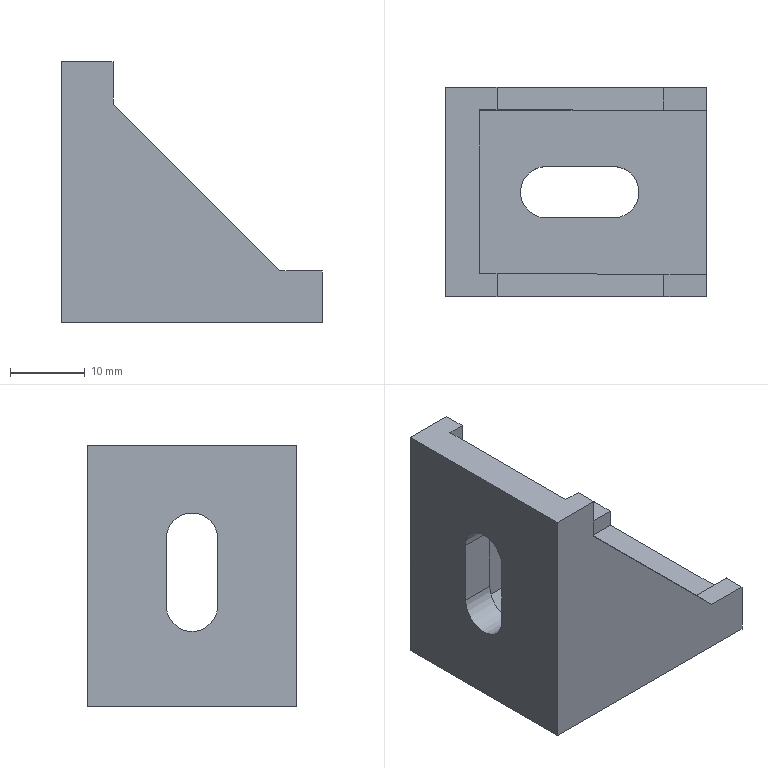Part | NX | features DATUM_CSYS 6, SKETCH 5, EXTRACT_DATUM_AXIS 4, EXTRACT_FACE 4, EXTRACT_STRING 4, EXTRUDE 4, Instance Feature 2, Mirror Feature 1, Pattern Feature 1, Variational Failed Derived Feature With Body 1 | 1 solid | 24 faces | box 35 x 28 x 35 mm | volume 9798 mm3 | plane 20 | cylinder 4 | commonest cylinder face diameters 6.9 x4
STEP:
#1=CARTESIAN_POINT('',(0.,14.,0.));
#2=VERTEX_POINT('',#1);
#3=CARTESIAN_POINT('',(35.,14.,0.));
#4=VERTEX_POINT('',#3);
#5=CARTESIAN_POINT('',(0.,14.,0.));
#6=DIRECTION('',(1.,0.,0.));
#7=VECTOR('',#6,1000.);
#8=LINE('',#5,#7);
#9=EDGE_CURVE('',#2,#4,#8,.T.);
#10=ORIENTED_EDGE('',*,*,#9,.T.);
#11=CARTESIAN_POINT('',(35.,-14.,0.));
#12=VERTEX_POINT('',#11);
#13=CARTESIAN_POINT('',(35.,-14.,0.));
#14=DIRECTION('',(0.,1.,0.));
#15=VECTOR('',#14,1000.);
#16=LINE('',#13,#15);
#17=EDGE_CURVE('',#12,#4,#16,.T.);
#18=ORIENTED_EDGE('',*,*,#17,.F.);
#19=CARTESIAN_POINT('',(0.,-14.,0.));
#20=VERTEX_POINT('',#19);
#21=CARTESIAN_POINT('',(0.,-14.,0.));
#22=DIRECTION('',(1.,0.,0.));
#23=VECTOR('',#22,1000.);
#24=LINE('',#21,#23);
#25=EDGE_CURVE('',#20,#12,#24,.T.);
#26=ORIENTED_EDGE('',*,*,#25,.F.);
#27=CARTESIAN_POINT('',(0.,-14.,0.));
#28=DIRECTION('',(0.,1.,0.));
#29=VECTOR('',#28,1000.);
#30=LINE('',#27,#29);
#31=EDGE_CURVE('',#20,#2,#30,.T.);
#32=ORIENTED_EDGE('',*,*,#31,.T.);
#33=EDGE_LOOP('',(#10,#18,#26,#32));
#34=FACE_BOUND('',#33,.T.);
#35=CARTESIAN_POINT('',(13.5,3.45,0.));
#36=VERTEX_POINT('',#35);
#37=CARTESIAN_POINT('',(13.5,-3.45,0.));
#38=VERTEX_POINT('',#37);
#39=CARTESIAN_POINT('',(13.5,0.,0.));
#40=DIRECTION('',(0.,0.,1.));
#41=DIRECTION('',(0.,-1.,0.));
#42=AXIS2_PLACEMENT_3D('',#39,#40,#41);
#43=CIRCLE('',#42,3.45);
#44=EDGE_CURVE('',#36,#38,#43,.T.);
#45=ORIENTED_EDGE('',*,*,#44,.T.);
#46=CARTESIAN_POINT('',(22.5,-3.45,0.));
#47=VERTEX_POINT('',#46);
#48=CARTESIAN_POINT('',(13.5,-3.45,0.));
#49=DIRECTION('',(1.,0.,0.));
#50=VECTOR('',#49,1000.);
#51=LINE('',#48,#50);
#52=EDGE_CURVE('',#38,#47,#51,.T.);
#53=ORIENTED_EDGE('',*,*,#52,.T.);
#54=CARTESIAN_POINT('',(22.5,3.45,0.));
#55=VERTEX_POINT('',#54);
#56=CARTESIAN_POINT('',(22.5,0.,0.));
#57=DIRECTION('',(0.,0.,1.));
#58=DIRECTION('',(0.,-1.,0.));
#59=AXIS2_PLACEMENT_3D('',#56,#57,#58);
#60=CIRCLE('',#59,3.45);
#61=EDGE_CURVE('',#47,#55,#60,.T.);
#62=ORIENTED_EDGE('',*,*,#61,.T.);
#63=CARTESIAN_POINT('',(22.5,3.45,0.));
#64=DIRECTION('',(-1.,0.,0.));
#65=VECTOR('',#64,1000.);
#66=LINE('',#63,#65);
#67=EDGE_CURVE('',#55,#36,#66,.T.);
#68=ORIENTED_EDGE('',*,*,#67,.T.);
#69=EDGE_LOOP('',(#45,#53,#62,#68));
#70=FACE_BOUND('',#69,.T.);
#71=CARTESIAN_POINT('',(0.,-14.,0.));
#72=DIRECTION('',(0.,0.,1.));
#73=DIRECTION('',(1.,0.,0.));
#74=AXIS2_PLACEMENT_3D('',#71,#72,#73);
#75=PLANE('',#74);
#76=ADVANCED_FACE('',(#34,#70),#75,.F.);
#77=CARTESIAN_POINT('',(0.,14.,35.));
#78=VERTEX_POINT('',#77);
#79=CARTESIAN_POINT('',(0.,14.,35.));
#80=DIRECTION('',(0.,0.,-1.));
#81=VECTOR('',#80,1000.);
#82=LINE('',#79,#81);
#83=EDGE_CURVE('',#78,#2,#82,.T.);
#84=ORIENTED_EDGE('',*,*,#83,.T.);
#85=ORIENTED_EDGE('',*,*,#31,.F.);
#86=CARTESIAN_POINT('',(0.,-14.,35.));
#87=VERTEX_POINT('',#86);
#88=CARTESIAN_POINT('',(0.,-14.,35.));
#89=DIRECTION('',(0.,0.,-1.));
#90=VECTOR('',#89,1000.);
#91=LINE('',#88,#90);
#92=EDGE_CURVE('',#87,#20,#91,.T.);
#93=ORIENTED_EDGE('',*,*,#92,.F.);
#94=CARTESIAN_POINT('',(0.,-14.,35.));
#95=DIRECTION('',(0.,1.,0.));
#96=VECTOR('',#95,1000.);
#97=LINE('',#94,#96);
#98=EDGE_CURVE('',#87,#78,#97,.T.);
#99=ORIENTED_EDGE('',*,*,#98,.T.);
#100=EDGE_LOOP('',(#84,#85,#93,#99));
#101=FACE_BOUND('',#100,.T.);
#102=CARTESIAN_POINT('',(0.,-3.45,13.5));
#103=VERTEX_POINT('',#102);
#104=CARTESIAN_POINT('',(0.,-3.45,22.5));
#105=VERTEX_POINT('',#104);
#106=CARTESIAN_POINT('',(0.,-3.45,13.5));
#107=DIRECTION('',(0.,0.,1.));
#108=VECTOR('',#107,1000.);
#109=LINE('',#106,#108);
#110=EDGE_CURVE('',#103,#105,#109,.T.);
#111=ORIENTED_EDGE('',*,*,#110,.F.);
#112=CARTESIAN_POINT('',(0.,3.45,13.5));
#113=VERTEX_POINT('',#112);
#114=CARTESIAN_POINT('',(0.,0.,13.5));
#115=DIRECTION('',(-1.,0.,0.));
#116=DIRECTION('',(0.,-1.,0.));
#117=AXIS2_PLACEMENT_3D('',#114,#115,#116);
#118=CIRCLE('',#117,3.45);
#119=EDGE_CURVE('',#113,#103,#118,.T.);
#120=ORIENTED_EDGE('',*,*,#119,.F.);
#121=CARTESIAN_POINT('',(0.,3.45,22.5));
#122=VERTEX_POINT('',#121);
#123=CARTESIAN_POINT('',(0.,3.45,22.5));
#124=DIRECTION('',(0.,0.,-1.));
#125=VECTOR('',#124,1000.);
#126=LINE('',#123,#125);
#127=EDGE_CURVE('',#122,#113,#126,.T.);
#128=ORIENTED_EDGE('',*,*,#127,.F.);
#129=CARTESIAN_POINT('',(0.,0.,22.5));
#130=DIRECTION('',(-1.,0.,0.));
#131=DIRECTION('',(0.,-1.,0.));
#132=AXIS2_PLACEMENT_3D('',#129,#130,#131);
#133=CIRCLE('',#132,3.45);
#134=EDGE_CURVE('',#105,#122,#133,.T.);
#135=ORIENTED_EDGE('',*,*,#134,.F.);
#136=EDGE_LOOP('',(#111,#120,#128,#135));
#137=FACE_BOUND('',#136,.T.);
#138=CARTESIAN_POINT('',(0.,-14.,35.));
#139=DIRECTION('',(1.,0.,0.));
#140=DIRECTION('',(0.,0.,-1.));
#141=AXIS2_PLACEMENT_3D('',#138,#139,#140);
#142=PLANE('',#141);
#143=ADVANCED_FACE('',(#101,#137),#142,.F.);
#144=CARTESIAN_POINT('',(6.9,11.,35.));
#145=VERTEX_POINT('',#144);
#146=CARTESIAN_POINT('',(4.58,11.,35.));
#147=VERTEX_POINT('',#146);
#148=CARTESIAN_POINT('',(35.,11.,35.));
#149=DIRECTION('',(-1.,0.,0.));
#150=VECTOR('',#149,1000.);
#151=LINE('',#148,#150);
#152=EDGE_CURVE('',#145,#147,#151,.T.);
#153=ORIENTED_EDGE('',*,*,#152,.F.);
#154=CARTESIAN_POINT('',(6.9,14.,35.));
#155=VERTEX_POINT('',#154);
#156=CARTESIAN_POINT('',(6.9,-14.,35.));
#157=DIRECTION('',(0.,1.,0.));
#158=VECTOR('',#157,1000.);
#159=LINE('',#156,#158);
#160=EDGE_CURVE('',#145,#155,#159,.T.);
#161=ORIENTED_EDGE('',*,*,#160,.T.);
#162=CARTESIAN_POINT('',(6.9,14.,35.));
#163=DIRECTION('',(-1.,0.,0.));
#164=VECTOR('',#163,1000.);
#165=LINE('',#162,#164);
#166=EDGE_CURVE('',#155,#78,#165,.T.);
#167=ORIENTED_EDGE('',*,*,#166,.T.);
#168=ORIENTED_EDGE('',*,*,#98,.F.);
#169=CARTESIAN_POINT('',(6.9,-14.,35.));
#170=VERTEX_POINT('',#169);
#171=CARTESIAN_POINT('',(6.9,-14.,35.));
#172=DIRECTION('',(-1.,0.,0.));
#173=VECTOR('',#172,1000.);
#174=LINE('',#171,#173);
#175=EDGE_CURVE('',#170,#87,#174,.T.);
#176=ORIENTED_EDGE('',*,*,#175,.F.);
#177=CARTESIAN_POINT('',(6.9,-11.,35.));
#178=VERTEX_POINT('',#177);
#179=CARTESIAN_POINT('',(6.9,-14.,35.));
#180=DIRECTION('',(0.,1.,0.));
#181=VECTOR('',#180,1000.);
#182=LINE('',#179,#181);
#183=EDGE_CURVE('',#170,#178,#182,.T.);
#184=ORIENTED_EDGE('',*,*,#183,.T.);
#185=CARTESIAN_POINT('',(4.58,-11.,35.));
#186=VERTEX_POINT('',#185);
#187=CARTESIAN_POINT('',(35.,-11.,35.));
#188=DIRECTION('',(-1.,0.,0.));
#189=VECTOR('',#188,1000.);
#190=LINE('',#187,#189);
#191=EDGE_CURVE('',#178,#186,#190,.T.);
#192=ORIENTED_EDGE('',*,*,#191,.T.);
#193=CARTESIAN_POINT('',(4.58,-11.,35.));
#194=DIRECTION('',(0.,1.,0.));
#195=VECTOR('',#194,1000.);
#196=LINE('',#193,#195);
#197=EDGE_CURVE('',#186,#147,#196,.T.);
#198=ORIENTED_EDGE('',*,*,#197,.T.);
#199=EDGE_LOOP('',(#153,#161,#167,#168,#176,#184,#192,#198));
#200=FACE_BOUND('',#199,.T.);
#201=CARTESIAN_POINT('',(6.9,-14.,35.));
#202=DIRECTION('',(0.,0.,-1.));
#203=DIRECTION('',(-1.,0.,0.));
#204=AXIS2_PLACEMENT_3D('',#201,#202,#203);
#205=PLANE('',#204);
#206=ADVANCED_FACE('',(#200),#205,.F.);
#207=CARTESIAN_POINT('',(35.,11.,4.58));
#208=VERTEX_POINT('',#207);
#209=CARTESIAN_POINT('',(35.,11.,6.9));
#210=VERTEX_POINT('',#209);
#211=CARTESIAN_POINT('',(35.,11.,4.58));
#212=DIRECTION('',(0.,0.,1.));
#213=VECTOR('',#212,1000.);
#214=LINE('',#211,#213);
#215=EDGE_CURVE('',#208,#210,#214,.T.);
#216=ORIENTED_EDGE('',*,*,#215,.F.);
#217=CARTESIAN_POINT('',(35.,-11.,4.58));
#218=VERTEX_POINT('',#217);
#219=CARTESIAN_POINT('',(35.,-11.,4.58));
#220=DIRECTION('',(0.,1.,0.));
#221=VECTOR('',#220,1000.);
#222=LINE('',#219,#221);
#223=EDGE_CURVE('',#218,#208,#222,.T.);
#224=ORIENTED_EDGE('',*,*,#223,.F.);
#225=CARTESIAN_POINT('',(35.,-11.,6.9));
#226=VERTEX_POINT('',#225);
#227=CARTESIAN_POINT('',(35.,-11.,4.58));
#228=DIRECTION('',(0.,0.,1.));
#229=VECTOR('',#228,1000.);
#230=LINE('',#227,#229);
#231=EDGE_CURVE('',#218,#226,#230,.T.);
#232=ORIENTED_EDGE('',*,*,#231,.T.);
#233=CARTESIAN_POINT('',(35.,-14.,6.9));
#234=VERTEX_POINT('',#233);
#235=CARTESIAN_POINT('',(35.,-14.,6.9));
#236=DIRECTION('',(0.,1.,0.));
#237=VECTOR('',#236,1000.);
#238=LINE('',#235,#237);
#239=EDGE_CURVE('',#234,#226,#238,.T.);
#240=ORIENTED_EDGE('',*,*,#239,.F.);
#241=CARTESIAN_POINT('',(35.,-14.,0.));
#242=DIRECTION('',(0.,0.,1.));
#243=VECTOR('',#242,1000.);
#244=LINE('',#241,#243);
#245=EDGE_CURVE('',#12,#234,#244,.T.);
#246=ORIENTED_EDGE('',*,*,#245,.F.);
#247=ORIENTED_EDGE('',*,*,#17,.T.);
#248=CARTESIAN_POINT('',(35.,14.,6.9));
#249=VERTEX_POINT('',#248);
#250=CARTESIAN_POINT('',(35.,14.,0.));
#251=DIRECTION('',(0.,0.,1.));
#252=VECTOR('',#251,1000.);
#253=LINE('',#250,#252);
#254=EDGE_CURVE('',#4,#249,#253,.T.);
#255=ORIENTED_EDGE('',*,*,#254,.T.);
#256=CARTESIAN_POINT('',(35.,-14.,6.9));
#257=DIRECTION('',(0.,1.,0.));
#258=VECTOR('',#257,1000.);
#259=LINE('',#256,#258);
#260=EDGE_CURVE('',#210,#249,#259,.T.);
#261=ORIENTED_EDGE('',*,*,#260,.F.);
#262=EDGE_LOOP('',(#216,#224,#232,#240,#246,#247,#255,#261));
#263=FACE_BOUND('',#262,.T.);
#264=CARTESIAN_POINT('',(35.,-14.,0.));
#265=DIRECTION('',(-1.,0.,0.));
#266=DIRECTION('',(0.,0.,1.));
#267=AXIS2_PLACEMENT_3D('',#264,#265,#266);
#268=PLANE('',#267);
#269=ADVANCED_FACE('',(#263),#268,.F.);
#270=CARTESIAN_POINT('',(29.3,11.,6.9));
#271=VERTEX_POINT('',#270);
#272=CARTESIAN_POINT('',(35.,11.,6.9));
#273=DIRECTION('',(-1.,0.,0.));
#274=VECTOR('',#273,1000.);
#275=LINE('',#272,#274);
#276=EDGE_CURVE('',#210,#271,#275,.T.);
#277=ORIENTED_EDGE('',*,*,#276,.F.);
#278=ORIENTED_EDGE('',*,*,#260,.T.);
#279=CARTESIAN_POINT('',(29.3,14.,6.9));
#280=VERTEX_POINT('',#279);
#281=CARTESIAN_POINT('',(35.,14.,6.9));
#282=DIRECTION('',(-1.,0.,0.));
#283=VECTOR('',#282,1000.);
#284=LINE('',#281,#283);
#285=EDGE_CURVE('',#249,#280,#284,.T.);
#286=ORIENTED_EDGE('',*,*,#285,.T.);
#287=CARTESIAN_POINT('',(29.3,-14.,6.9));
#288=DIRECTION('',(0.,1.,0.));
#289=VECTOR('',#288,1000.);
#290=LINE('',#287,#289);
#291=EDGE_CURVE('',#271,#280,#290,.T.);
#292=ORIENTED_EDGE('',*,*,#291,.F.);
#293=EDGE_LOOP('',(#277,#278,#286,#292));
#294=FACE_BOUND('',#293,.T.);
#295=CARTESIAN_POINT('',(35.,-14.,6.9));
#296=DIRECTION('',(0.,0.,-1.));
#297=DIRECTION('',(-1.,0.,0.));
#298=AXIS2_PLACEMENT_3D('',#295,#296,#297);
#299=PLANE('',#298);
#300=ADVANCED_FACE('',(#294),#299,.F.);
#301=CARTESIAN_POINT('',(6.9,11.,29.3));
#302=VERTEX_POINT('',#301);
#303=CARTESIAN_POINT('',(29.3,11.,6.9));
#304=DIRECTION('',(-0.7071,0.,0.7071));
#305=VECTOR('',#304,1000.);
#306=LINE('',#303,#305);
#307=EDGE_CURVE('',#271,#302,#306,.T.);
#308=ORIENTED_EDGE('',*,*,#307,.F.);
#309=ORIENTED_EDGE('',*,*,#291,.T.);
#310=CARTESIAN_POINT('',(6.9,14.,29.3));
#311=VERTEX_POINT('',#310);
#312=CARTESIAN_POINT('',(29.3,14.,6.9));
#313=DIRECTION('',(-0.7071,0.,0.7071));
#314=VECTOR('',#313,1000.);
#315=LINE('',#312,#314);
#316=EDGE_CURVE('',#280,#311,#315,.T.);
#317=ORIENTED_EDGE('',*,*,#316,.T.);
#318=CARTESIAN_POINT('',(6.9,-14.,29.3));
#319=DIRECTION('',(0.,1.,0.));
#320=VECTOR('',#319,1000.);
#321=LINE('',#318,#320);
#322=EDGE_CURVE('',#302,#311,#321,.T.);
#323=ORIENTED_EDGE('',*,*,#322,.F.);
#324=EDGE_LOOP('',(#308,#309,#317,#323));
#325=FACE_BOUND('',#324,.T.);
#326=CARTESIAN_POINT('',(29.3,-14.,6.9));
#327=DIRECTION('',(-0.7071,0.,-0.7071));
#328=DIRECTION('',(-0.7071,0.,0.7071));
#329=AXIS2_PLACEMENT_3D('',#326,#327,#328);
#330=PLANE('',#329);
#331=ADVANCED_FACE('',(#325),#330,.F.);
#332=CARTESIAN_POINT('',(6.9,11.,29.3));
#333=DIRECTION('',(0.,0.,1.));
#334=VECTOR('',#333,1000.);
#335=LINE('',#332,#334);
#336=EDGE_CURVE('',#302,#145,#335,.T.);
#337=ORIENTED_EDGE('',*,*,#336,.F.);
#338=ORIENTED_EDGE('',*,*,#322,.T.);
#339=CARTESIAN_POINT('',(6.9,14.,29.3));
#340=DIRECTION('',(0.,0.,1.));
#341=VECTOR('',#340,1000.);
#342=LINE('',#339,#341);
#343=EDGE_CURVE('',#311,#155,#342,.T.);
#344=ORIENTED_EDGE('',*,*,#343,.T.);
#345=ORIENTED_EDGE('',*,*,#160,.F.);
#346=EDGE_LOOP('',(#337,#338,#344,#345));
#347=FACE_BOUND('',#346,.T.);
#348=CARTESIAN_POINT('',(6.9,-14.,29.3));
#349=DIRECTION('',(-1.,0.,0.));
#350=DIRECTION('',(0.,0.,1.));
#351=AXIS2_PLACEMENT_3D('',#348,#349,#350);
#352=PLANE('',#351);
#353=ADVANCED_FACE('',(#347),#352,.F.);
#354=ORIENTED_EDGE('',*,*,#239,.T.);
#355=CARTESIAN_POINT('',(29.3,-11.,6.9));
#356=VERTEX_POINT('',#355);
#357=CARTESIAN_POINT('',(35.,-11.,6.9));
#358=DIRECTION('',(-1.,0.,0.));
#359=VECTOR('',#358,1000.);
#360=LINE('',#357,#359);
#361=EDGE_CURVE('',#226,#356,#360,.T.);
#362=ORIENTED_EDGE('',*,*,#361,.T.);
#363=CARTESIAN_POINT('',(29.3,-14.,6.9));
#364=VERTEX_POINT('',#363);
#365=CARTESIAN_POINT('',(29.3,-14.,6.9));
#366=DIRECTION('',(0.,1.,0.));
#367=VECTOR('',#366,1000.);
#368=LINE('',#365,#367);
#369=EDGE_CURVE('',#364,#356,#368,.T.);
#370=ORIENTED_EDGE('',*,*,#369,.F.);
#371=CARTESIAN_POINT('',(35.,-14.,6.9));
#372=DIRECTION('',(-1.,0.,0.));
#373=VECTOR('',#372,1000.);
#374=LINE('',#371,#373);
#375=EDGE_CURVE('',#234,#364,#374,.T.);
#376=ORIENTED_EDGE('',*,*,#375,.F.);
#377=EDGE_LOOP('',(#354,#362,#370,#376));
#378=FACE_BOUND('',#377,.T.);
#379=CARTESIAN_POINT('',(35.,-14.,6.9));
#380=DIRECTION('',(0.,0.,-1.));
#381=DIRECTION('',(-1.,0.,0.));
#382=AXIS2_PLACEMENT_3D('',#379,#380,#381);
#383=PLANE('',#382);
#384=ADVANCED_FACE('',(#378),#383,.F.);
#385=ORIENTED_EDGE('',*,*,#369,.T.);
#386=CARTESIAN_POINT('',(6.9,-11.,29.3));
#387=VERTEX_POINT('',#386);
#388=CARTESIAN_POINT('',(29.3,-11.,6.9));
#389=DIRECTION('',(-0.7071,0.,0.7071));
#390=VECTOR('',#389,1000.);
#391=LINE('',#388,#390);
#392=EDGE_CURVE('',#356,#387,#391,.T.);
#393=ORIENTED_EDGE('',*,*,#392,.T.);
#394=CARTESIAN_POINT('',(6.9,-14.,29.3));
#395=VERTEX_POINT('',#394);
#396=CARTESIAN_POINT('',(6.9,-14.,29.3));
#397=DIRECTION('',(0.,1.,0.));
#398=VECTOR('',#397,1000.);
#399=LINE('',#396,#398);
#400=EDGE_CURVE('',#395,#387,#399,.T.);
#401=ORIENTED_EDGE('',*,*,#400,.F.);
#402=CARTESIAN_POINT('',(29.3,-14.,6.9));
#403=DIRECTION('',(-0.7071,0.,0.7071));
#404=VECTOR('',#403,1000.);
#405=LINE('',#402,#404);
#406=EDGE_CURVE('',#364,#395,#405,.T.);
#407=ORIENTED_EDGE('',*,*,#406,.F.);
#408=EDGE_LOOP('',(#385,#393,#401,#407));
#409=FACE_BOUND('',#408,.T.);
#410=CARTESIAN_POINT('',(29.3,-14.,6.9));
#411=DIRECTION('',(-0.7071,0.,-0.7071));
#412=DIRECTION('',(-0.7071,0.,0.7071));
#413=AXIS2_PLACEMENT_3D('',#410,#411,#412);
#414=PLANE('',#413);
#415=ADVANCED_FACE('',(#409),#414,.F.);
#416=ORIENTED_EDGE('',*,*,#400,.T.);
#417=CARTESIAN_POINT('',(6.9,-11.,29.3));
#418=DIRECTION('',(0.,0.,1.));
#419=VECTOR('',#418,1000.);
#420=LINE('',#417,#419);
#421=EDGE_CURVE('',#387,#178,#420,.T.);
#422=ORIENTED_EDGE('',*,*,#421,.T.);
#423=ORIENTED_EDGE('',*,*,#183,.F.);
#424=CARTESIAN_POINT('',(6.9,-14.,29.3));
#425=DIRECTION('',(0.,0.,1.));
#426=VECTOR('',#425,1000.);
#427=LINE('',#424,#426);
#428=EDGE_CURVE('',#395,#170,#427,.T.);
#429=ORIENTED_EDGE('',*,*,#428,.F.);
#430=EDGE_LOOP('',(#416,#422,#423,#429));
#431=FACE_BOUND('',#430,.T.);
#432=CARTESIAN_POINT('',(6.9,-14.,29.3));
#433=DIRECTION('',(-1.,0.,0.));
#434=DIRECTION('',(0.,0.,1.));
#435=AXIS2_PLACEMENT_3D('',#432,#433,#434);
#436=PLANE('',#435);
#437=ADVANCED_FACE('',(#431),#436,.F.);
#438=ORIENTED_EDGE('',*,*,#375,.T.);
#439=ORIENTED_EDGE('',*,*,#406,.T.);
#440=ORIENTED_EDGE('',*,*,#428,.T.);
#441=ORIENTED_EDGE('',*,*,#175,.T.);
#442=ORIENTED_EDGE('',*,*,#92,.T.);
#443=ORIENTED_EDGE('',*,*,#25,.T.);
#444=ORIENTED_EDGE('',*,*,#245,.T.);
#445=EDGE_LOOP('',(#438,#439,#440,#441,#442,#443,#444));
#446=FACE_BOUND('',#445,.T.);
#447=CARTESIAN_POINT('',(0.,-14.,0.));
#448=DIRECTION('',(0.,1.,0.));
#449=DIRECTION('',(0.,0.,1.));
#450=AXIS2_PLACEMENT_3D('',#447,#448,#449);
#451=PLANE('',#450);
#452=ADVANCED_FACE('',(#446),#451,.F.);
#453=ORIENTED_EDGE('',*,*,#285,.F.);
#454=ORIENTED_EDGE('',*,*,#254,.F.);
#455=ORIENTED_EDGE('',*,*,#9,.F.);
#456=ORIENTED_EDGE('',*,*,#83,.F.);
#457=ORIENTED_EDGE('',*,*,#166,.F.);
#458=ORIENTED_EDGE('',*,*,#343,.F.);
#459=ORIENTED_EDGE('',*,*,#316,.F.);
#460=EDGE_LOOP('',(#453,#454,#455,#456,#457,#458,#459));
#461=FACE_BOUND('',#460,.T.);
#462=CARTESIAN_POINT('',(0.,14.,0.));
#463=DIRECTION('',(0.,1.,0.));
#464=DIRECTION('',(0.,0.,1.));
#465=AXIS2_PLACEMENT_3D('',#462,#463,#464);
#466=PLANE('',#465);
#467=ADVANCED_FACE('',(#461),#466,.T.);
#468=ORIENTED_EDGE('',*,*,#231,.F.);
#469=CARTESIAN_POINT('',(4.58,-11.,4.58));
#470=VERTEX_POINT('',#469);
#471=CARTESIAN_POINT('',(4.58,-11.,4.58));
#472=DIRECTION('',(1.,0.,0.));
#473=VECTOR('',#472,1000.);
#474=LINE('',#471,#473);
#475=EDGE_CURVE('',#218,#470,#474,.F.);
#476=ORIENTED_EDGE('',*,*,#475,.T.);
#477=CARTESIAN_POINT('',(4.58,-11.,35.));
#478=DIRECTION('',(0.,0.,-1.));
#479=VECTOR('',#478,1000.);
#480=LINE('',#477,#479);
#481=EDGE_CURVE('',#470,#186,#480,.F.);
#482=ORIENTED_EDGE('',*,*,#481,.T.);
#483=ORIENTED_EDGE('',*,*,#191,.F.);
#484=ORIENTED_EDGE('',*,*,#421,.F.);
#485=ORIENTED_EDGE('',*,*,#392,.F.);
#486=ORIENTED_EDGE('',*,*,#361,.F.);
#487=EDGE_LOOP('',(#468,#476,#482,#483,#484,#485,#486));
#488=FACE_BOUND('',#487,.T.);
#489=CARTESIAN_POINT('',(0.,-11.,0.));
#490=DIRECTION('',(0.,-1.,0.));
#491=DIRECTION('',(0.,0.,-1.));
#492=AXIS2_PLACEMENT_3D('',#489,#490,#491);
#493=PLANE('',#492);
#494=ADVANCED_FACE('',(#488),#493,.F.);
#495=ORIENTED_EDGE('',*,*,#276,.T.);
#496=ORIENTED_EDGE('',*,*,#307,.T.);
#497=ORIENTED_EDGE('',*,*,#336,.T.);
#498=ORIENTED_EDGE('',*,*,#152,.T.);
#499=CARTESIAN_POINT('',(4.58,11.,4.58));
#500=VERTEX_POINT('',#499);
#501=CARTESIAN_POINT('',(4.58,11.,35.));
#502=DIRECTION('',(0.,0.,-1.));
#503=VECTOR('',#502,1000.);
#504=LINE('',#501,#503);
#505=EDGE_CURVE('',#500,#147,#504,.F.);
#506=ORIENTED_EDGE('',*,*,#505,.F.);
#507=CARTESIAN_POINT('',(4.58,11.,4.58));
#508=DIRECTION('',(1.,0.,0.));
#509=VECTOR('',#508,1000.);
#510=LINE('',#507,#509);
#511=EDGE_CURVE('',#208,#500,#510,.F.);
#512=ORIENTED_EDGE('',*,*,#511,.F.);
#513=ORIENTED_EDGE('',*,*,#215,.T.);
#514=EDGE_LOOP('',(#495,#496,#497,#498,#506,#512,#513));
#515=FACE_BOUND('',#514,.T.);
#516=CARTESIAN_POINT('',(0.,11.,0.));
#517=DIRECTION('',(0.,-1.,0.));
#518=DIRECTION('',(0.,0.,-1.));
#519=AXIS2_PLACEMENT_3D('',#516,#517,#518);
#520=PLANE('',#519);
#521=ADVANCED_FACE('',(#515),#520,.T.);
#522=CARTESIAN_POINT('',(4.58,-3.45,22.5));
#523=VERTEX_POINT('',#522);
#524=CARTESIAN_POINT('',(4.58,-3.45,13.5));
#525=VERTEX_POINT('',#524);
#526=CARTESIAN_POINT('',(4.58,-3.45,35.));
#527=DIRECTION('',(0.,0.,-1.));
#528=VECTOR('',#527,1000.);
#529=LINE('',#526,#528);
#530=EDGE_CURVE('',#523,#525,#529,.T.);
#531=ORIENTED_EDGE('',*,*,#530,.F.);
#532=CARTESIAN_POINT('',(4.58,3.45,22.5));
#533=VERTEX_POINT('',#532);
#534=CARTESIAN_POINT('',(4.58,0.,22.5));
#535=DIRECTION('',(1.,0.,0.));
#536=DIRECTION('',(0.,0.,-1.));
#537=AXIS2_PLACEMENT_3D('',#534,#535,#536);
#538=CIRCLE('',#537,3.45);
#539=EDGE_CURVE('',#533,#523,#538,.T.);
#540=ORIENTED_EDGE('',*,*,#539,.F.);
#541=CARTESIAN_POINT('',(4.58,3.45,13.5));
#542=VERTEX_POINT('',#541);
#543=CARTESIAN_POINT('',(4.58,3.45,35.));
#544=DIRECTION('',(0.,0.,1.));
#545=VECTOR('',#544,1000.);
#546=LINE('',#543,#545);
#547=EDGE_CURVE('',#542,#533,#546,.T.);
#548=ORIENTED_EDGE('',*,*,#547,.F.);
#549=CARTESIAN_POINT('',(4.58,0.,13.5));
#550=DIRECTION('',(1.,0.,0.));
#551=DIRECTION('',(0.,0.,-1.));
#552=AXIS2_PLACEMENT_3D('',#549,#550,#551);
#553=CIRCLE('',#552,3.45);
#554=EDGE_CURVE('',#525,#542,#553,.T.);
#555=ORIENTED_EDGE('',*,*,#554,.F.);
#556=EDGE_LOOP('',(#531,#540,#548,#555));
#557=FACE_BOUND('',#556,.T.);
#558=ORIENTED_EDGE('',*,*,#505,.T.);
#559=ORIENTED_EDGE('',*,*,#197,.F.);
#560=ORIENTED_EDGE('',*,*,#481,.F.);
#561=CARTESIAN_POINT('',(4.58,-11.,4.58));
#562=DIRECTION('',(0.,1.,0.));
#563=VECTOR('',#562,1000.);
#564=LINE('',#561,#563);
#565=EDGE_CURVE('',#500,#470,#564,.F.);
#566=ORIENTED_EDGE('',*,*,#565,.F.);
#567=EDGE_LOOP('',(#558,#559,#560,#566));
#568=FACE_BOUND('',#567,.T.);
#569=CARTESIAN_POINT('',(4.58,-11.,35.));
#570=DIRECTION('',(1.,0.,0.));
#571=DIRECTION('',(0.,0.,-1.));
#572=AXIS2_PLACEMENT_3D('',#569,#570,#571);
#573=PLANE('',#572);
#574=ADVANCED_FACE('',(#557,#568),#573,.T.);
#575=CARTESIAN_POINT('',(22.5,3.45,4.58));
#576=VERTEX_POINT('',#575);
#577=CARTESIAN_POINT('',(22.5,-3.45,4.58));
#578=VERTEX_POINT('',#577);
#579=CARTESIAN_POINT('',(22.5,0.,4.58));
#580=DIRECTION('',(0.,0.,1.));
#581=DIRECTION('',(1.,0.,0.));
#582=AXIS2_PLACEMENT_3D('',#579,#580,#581);
#583=CIRCLE('',#582,3.45);
#584=EDGE_CURVE('',#576,#578,#583,.F.);
#585=ORIENTED_EDGE('',*,*,#584,.T.);
#586=CARTESIAN_POINT('',(13.5,-3.45,4.58));
#587=VERTEX_POINT('',#586);
#588=CARTESIAN_POINT('',(4.58,-3.45,4.58));
#589=DIRECTION('',(-1.,0.,0.));
#590=VECTOR('',#589,1000.);
#591=LINE('',#588,#590);
#592=EDGE_CURVE('',#578,#587,#591,.T.);
#593=ORIENTED_EDGE('',*,*,#592,.T.);
#594=CARTESIAN_POINT('',(13.5,3.45,4.58));
#595=VERTEX_POINT('',#594);
#596=CARTESIAN_POINT('',(13.5,0.,4.58));
#597=DIRECTION('',(0.,0.,1.));
#598=DIRECTION('',(1.,0.,0.));
#599=AXIS2_PLACEMENT_3D('',#596,#597,#598);
#600=CIRCLE('',#599,3.45);
#601=EDGE_CURVE('',#587,#595,#600,.F.);
#602=ORIENTED_EDGE('',*,*,#601,.T.);
#603=CARTESIAN_POINT('',(4.58,3.45,4.58));
#604=DIRECTION('',(1.,0.,0.));
#605=VECTOR('',#604,1000.);
#606=LINE('',#603,#605);
#607=EDGE_CURVE('',#595,#576,#606,.T.);
#608=ORIENTED_EDGE('',*,*,#607,.T.);
#609=EDGE_LOOP('',(#585,#593,#602,#608));
#610=FACE_BOUND('',#609,.T.);
#611=ORIENTED_EDGE('',*,*,#511,.T.);
#612=ORIENTED_EDGE('',*,*,#565,.T.);
#613=ORIENTED_EDGE('',*,*,#475,.F.);
#614=ORIENTED_EDGE('',*,*,#223,.T.);
#615=EDGE_LOOP('',(#611,#612,#613,#614));
#616=FACE_BOUND('',#615,.T.);
#617=CARTESIAN_POINT('',(4.58,-11.,4.58));
#618=DIRECTION('',(0.,0.,1.));
#619=DIRECTION('',(1.,0.,0.));
#620=AXIS2_PLACEMENT_3D('',#617,#618,#619);
#621=PLANE('',#620);
#622=ADVANCED_FACE('',(#610,#616),#621,.T.);
#623=ORIENTED_EDGE('',*,*,#530,.T.);
#624=CARTESIAN_POINT('',(38.5,-3.45,13.5));
#625=DIRECTION('',(-1.,0.,0.));
#626=VECTOR('',#625,1000.);
#627=LINE('',#624,#626);
#628=EDGE_CURVE('',#103,#525,#627,.F.);
#629=ORIENTED_EDGE('',*,*,#628,.F.);
#630=ORIENTED_EDGE('',*,*,#110,.T.);
#631=CARTESIAN_POINT('',(38.5,-3.45,22.5));
#632=DIRECTION('',(-1.,0.,0.));
#633=VECTOR('',#632,1000.);
#634=LINE('',#631,#633);
#635=EDGE_CURVE('',#105,#523,#634,.F.);
#636=ORIENTED_EDGE('',*,*,#635,.T.);
#637=EDGE_LOOP('',(#623,#629,#630,#636));
#638=FACE_BOUND('',#637,.T.);
#639=CARTESIAN_POINT('',(38.5,-3.45,13.5));
#640=DIRECTION('',(0.,-1.,0.));
#641=DIRECTION('',(0.,0.,-1.));
#642=AXIS2_PLACEMENT_3D('',#639,#640,#641);
#643=PLANE('',#642);
#644=ADVANCED_FACE('',(#638),#643,.F.);
#645=ORIENTED_EDGE('',*,*,#539,.T.);
#646=ORIENTED_EDGE('',*,*,#635,.F.);
#647=ORIENTED_EDGE('',*,*,#134,.T.);
#648=CARTESIAN_POINT('',(38.5,3.45,22.5));
#649=DIRECTION('',(-1.,0.,0.));
#650=VECTOR('',#649,1000.);
#651=LINE('',#648,#650);
#652=EDGE_CURVE('',#122,#533,#651,.F.);
#653=ORIENTED_EDGE('',*,*,#652,.T.);
#654=EDGE_LOOP('',(#645,#646,#647,#653));
#655=FACE_BOUND('',#654,.T.);
#656=CARTESIAN_POINT('',(38.5,0.,22.5));
#657=DIRECTION('',(-1.,0.,0.));
#658=DIRECTION('',(0.,0.,1.));
#659=AXIS2_PLACEMENT_3D('',#656,#657,#658);
#660=CYLINDRICAL_SURFACE('',#659,3.45);
#661=ADVANCED_FACE('',(#655),#660,.F.);
#662=ORIENTED_EDGE('',*,*,#547,.T.);
#663=ORIENTED_EDGE('',*,*,#652,.F.);
#664=ORIENTED_EDGE('',*,*,#127,.T.);
#665=CARTESIAN_POINT('',(38.5,3.45,13.5));
#666=DIRECTION('',(-1.,0.,0.));
#667=VECTOR('',#666,1000.);
#668=LINE('',#665,#667);
#669=EDGE_CURVE('',#113,#542,#668,.F.);
#670=ORIENTED_EDGE('',*,*,#669,.T.);
#671=EDGE_LOOP('',(#662,#663,#664,#670));
#672=FACE_BOUND('',#671,.T.);
#673=CARTESIAN_POINT('',(38.5,3.45,22.5));
#674=DIRECTION('',(0.,1.,0.));
#675=DIRECTION('',(0.,0.,1.));
#676=AXIS2_PLACEMENT_3D('',#673,#674,#675);
#677=PLANE('',#676);
#678=ADVANCED_FACE('',(#672),#677,.F.);
#679=ORIENTED_EDGE('',*,*,#554,.T.);
#680=ORIENTED_EDGE('',*,*,#669,.F.);
#681=ORIENTED_EDGE('',*,*,#119,.T.);
#682=ORIENTED_EDGE('',*,*,#628,.T.);
#683=EDGE_LOOP('',(#679,#680,#681,#682));
#684=FACE_BOUND('',#683,.T.);
#685=CARTESIAN_POINT('',(38.5,0.,13.5));
#686=DIRECTION('',(-1.,0.,0.));
#687=DIRECTION('',(0.,0.,1.));
#688=AXIS2_PLACEMENT_3D('',#685,#686,#687);
#689=CYLINDRICAL_SURFACE('',#688,3.45);
#690=ADVANCED_FACE('',(#684),#689,.F.);
#691=CARTESIAN_POINT('',(22.5,-3.45,38.5));
#692=DIRECTION('',(0.,0.,-1.));
#693=VECTOR('',#692,1000.);
#694=LINE('',#691,#693);
#695=EDGE_CURVE('',#47,#578,#694,.F.);
#696=ORIENTED_EDGE('',*,*,#695,.F.);
#697=ORIENTED_EDGE('',*,*,#52,.F.);
#698=CARTESIAN_POINT('',(13.5,-3.45,38.5));
#699=DIRECTION('',(0.,0.,-1.));
#700=VECTOR('',#699,1000.);
#701=LINE('',#698,#700);
#702=EDGE_CURVE('',#38,#587,#701,.F.);
#703=ORIENTED_EDGE('',*,*,#702,.T.);
#704=ORIENTED_EDGE('',*,*,#592,.F.);
#705=EDGE_LOOP('',(#696,#697,#703,#704));
#706=FACE_BOUND('',#705,.T.);
#707=CARTESIAN_POINT('',(13.5,-3.45,38.5));
#708=DIRECTION('',(0.,1.,0.));
#709=DIRECTION('',(0.,0.,1.));
#710=AXIS2_PLACEMENT_3D('',#707,#708,#709);
#711=PLANE('',#710);
#712=ADVANCED_FACE('',(#706),#711,.T.);
#713=CARTESIAN_POINT('',(22.5,3.45,38.5));
#714=DIRECTION('',(0.,0.,-1.));
#715=VECTOR('',#714,1000.);
#716=LINE('',#713,#715);
#717=EDGE_CURVE('',#55,#576,#716,.F.);
#718=ORIENTED_EDGE('',*,*,#717,.F.);
#719=ORIENTED_EDGE('',*,*,#61,.F.);
#720=ORIENTED_EDGE('',*,*,#695,.T.);
#721=ORIENTED_EDGE('',*,*,#584,.F.);
#722=EDGE_LOOP('',(#718,#719,#720,#721));
#723=FACE_BOUND('',#722,.T.);
#724=CARTESIAN_POINT('',(22.5,0.,38.5));
#725=DIRECTION('',(0.,0.,-1.));
#726=DIRECTION('',(-1.,0.,0.));
#727=AXIS2_PLACEMENT_3D('',#724,#725,#726);
#728=CYLINDRICAL_SURFACE('',#727,3.45);
#729=ADVANCED_FACE('',(#723),#728,.F.);
#730=CARTESIAN_POINT('',(13.5,3.45,38.5));
#731=DIRECTION('',(0.,0.,-1.));
#732=VECTOR('',#731,1000.);
#733=LINE('',#730,#732);
#734=EDGE_CURVE('',#36,#595,#733,.F.);
#735=ORIENTED_EDGE('',*,*,#734,.F.);
#736=ORIENTED_EDGE('',*,*,#67,.F.);
#737=ORIENTED_EDGE('',*,*,#717,.T.);
#738=ORIENTED_EDGE('',*,*,#607,.F.);
#739=EDGE_LOOP('',(#735,#736,#737,#738));
#740=FACE_BOUND('',#739,.T.);
#741=CARTESIAN_POINT('',(22.5,3.45,38.5));
#742=DIRECTION('',(0.,-1.,0.));
#743=DIRECTION('',(1.,0.,0.));
#744=AXIS2_PLACEMENT_3D('',#741,#742,#743);
#745=PLANE('',#744);
#746=ADVANCED_FACE('',(#740),#745,.T.);
#747=ORIENTED_EDGE('',*,*,#702,.F.);
#748=ORIENTED_EDGE('',*,*,#44,.F.);
#749=ORIENTED_EDGE('',*,*,#734,.T.);
#750=ORIENTED_EDGE('',*,*,#601,.F.);
#751=EDGE_LOOP('',(#747,#748,#749,#750));
#752=FACE_BOUND('',#751,.T.);
#753=CARTESIAN_POINT('',(13.5,0.,38.5));
#754=DIRECTION('',(0.,0.,-1.));
#755=DIRECTION('',(-1.,0.,0.));
#756=AXIS2_PLACEMENT_3D('',#753,#754,#755);
#757=CYLINDRICAL_SURFACE('',#756,3.45);
#758=ADVANCED_FACE('',(#752),#757,.F.);
#759=CLOSED_SHELL('',(#76,#143,#206,#269,#300,#331,#353,#384,#415,#437,#452,#467,#494,#521,#574,#622,#644,#661,#678,#690,#712,#729,#746,#758));
#760=MANIFOLD_SOLID_BREP('',#759);
#761=(LENGTH_UNIT()NAMED_UNIT(*)SI_UNIT(.MILLI.,.METRE.));
#762=UNCERTAINTY_MEASURE_WITH_UNIT(LENGTH_MEASURE(0.00001),#761,'','');
#763=(NAMED_UNIT(*)PLANE_ANGLE_UNIT()SI_UNIT($,.RADIAN.));
#764=(NAMED_UNIT(*)SI_UNIT($,.STERADIAN.)SOLID_ANGLE_UNIT());
#765=(GEOMETRIC_REPRESENTATION_CONTEXT(3)GLOBAL_UNCERTAINTY_ASSIGNED_CONTEXT((#762))GLOBAL_UNIT_ASSIGNED_CONTEXT((#761,#763,#764))REPRESENTATION_CONTEXT('',''));
#766=ADVANCED_BREP_SHAPE_REPRESENTATION('',(#760),#765);